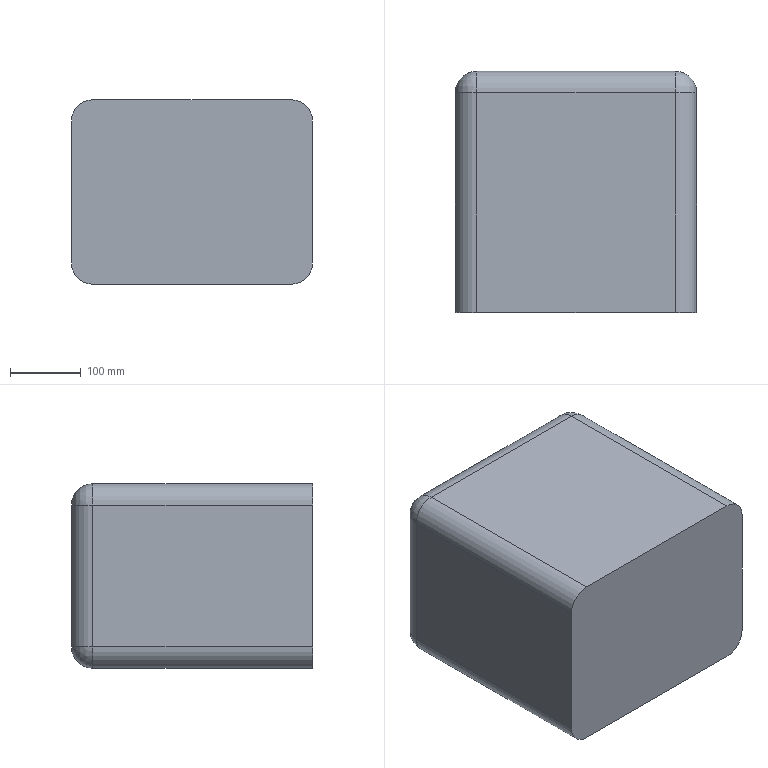Part | 1 solid | 18 faces | box 340 x 340 x 260 mm | volume 29579637 mm3 | cylinder 8 | plane 6 | sphere 4 | commonest cylinder face diameters 60 x8
STEP:
#1=CARTESIAN_POINT('',(170.,0.,100.));
#2=VERTEX_POINT('',#1);
#3=CARTESIAN_POINT('',(170.,0.,-100.));
#4=VERTEX_POINT('',#3);
#5=CARTESIAN_POINT('',(170.,0.,-130.));
#6=DIRECTION('',(0.,0.,-1.));
#7=VECTOR('',#6,1000.);
#8=LINE('',#5,#7);
#9=EDGE_CURVE('',#2,#4,#8,.T.);
#10=ORIENTED_EDGE('',*,*,#9,.T.);
#11=CARTESIAN_POINT('',(170.,310.,-100.));
#12=VERTEX_POINT('',#11);
#13=CARTESIAN_POINT('',(170.,340.,-100.));
#14=DIRECTION('',(0.,1.,0.));
#15=VECTOR('',#14,1000.);
#16=LINE('',#13,#15);
#17=EDGE_CURVE('',#4,#12,#16,.T.);
#18=ORIENTED_EDGE('',*,*,#17,.T.);
#19=CARTESIAN_POINT('',(170.,310.,100.));
#20=VERTEX_POINT('',#19);
#21=CARTESIAN_POINT('',(170.,310.,130.));
#22=DIRECTION('',(0.,0.,1.));
#23=VECTOR('',#22,1000.);
#24=LINE('',#21,#23);
#25=EDGE_CURVE('',#12,#20,#24,.T.);
#26=ORIENTED_EDGE('',*,*,#25,.T.);
#27=CARTESIAN_POINT('',(170.,340.,100.));
#28=DIRECTION('',(0.,-1.,0.));
#29=VECTOR('',#28,1000.);
#30=LINE('',#27,#29);
#31=EDGE_CURVE('',#20,#2,#30,.T.);
#32=ORIENTED_EDGE('',*,*,#31,.T.);
#33=EDGE_LOOP('',(#10,#18,#26,#32));
#34=FACE_OUTER_BOUND('',#33,.T.);
#35=CARTESIAN_POINT('',(170.,340.,-130.));
#36=DIRECTION('',(-1.,0.,0.));
#37=DIRECTION('',(0.,0.,1.));
#38=AXIS2_PLACEMENT_3D('',#35,#36,#37);
#39=PLANE('',#38);
#40=ADVANCED_FACE('',(#34),#39,.F.);
#41=CARTESIAN_POINT('',(140.,0.,-130.));
#42=VERTEX_POINT('',#41);
#43=CARTESIAN_POINT('',(-140.,0.,-130.));
#44=VERTEX_POINT('',#43);
#45=CARTESIAN_POINT('',(-170.,0.,-130.));
#46=DIRECTION('',(-1.,0.,0.));
#47=VECTOR('',#46,1000.);
#48=LINE('',#45,#47);
#49=EDGE_CURVE('',#42,#44,#48,.T.);
#50=ORIENTED_EDGE('',*,*,#49,.T.);
#51=CARTESIAN_POINT('',(-140.,310.,-130.));
#52=VERTEX_POINT('',#51);
#53=CARTESIAN_POINT('',(-140.,340.,-130.));
#54=DIRECTION('',(0.,1.,0.));
#55=VECTOR('',#54,1000.);
#56=LINE('',#53,#55);
#57=EDGE_CURVE('',#44,#52,#56,.T.);
#58=ORIENTED_EDGE('',*,*,#57,.T.);
#59=CARTESIAN_POINT('',(140.,310.,-130.));
#60=VERTEX_POINT('',#59);
#61=CARTESIAN_POINT('',(170.,310.,-130.));
#62=DIRECTION('',(1.,0.,0.));
#63=VECTOR('',#62,1000.);
#64=LINE('',#61,#63);
#65=EDGE_CURVE('',#52,#60,#64,.T.);
#66=ORIENTED_EDGE('',*,*,#65,.T.);
#67=CARTESIAN_POINT('',(140.,340.,-130.));
#68=DIRECTION('',(0.,-1.,0.));
#69=VECTOR('',#68,1000.);
#70=LINE('',#67,#69);
#71=EDGE_CURVE('',#60,#42,#70,.T.);
#72=ORIENTED_EDGE('',*,*,#71,.T.);
#73=EDGE_LOOP('',(#50,#58,#66,#72));
#74=FACE_OUTER_BOUND('',#73,.T.);
#75=CARTESIAN_POINT('',(-170.,340.,-130.));
#76=DIRECTION('',(0.,0.,1.));
#77=DIRECTION('',(1.,0.,0.));
#78=AXIS2_PLACEMENT_3D('',#75,#76,#77);
#79=PLANE('',#78);
#80=ADVANCED_FACE('',(#74),#79,.F.);
#81=CARTESIAN_POINT('',(-170.,310.,100.));
#82=VERTEX_POINT('',#81);
#83=CARTESIAN_POINT('',(-170.,310.,-100.));
#84=VERTEX_POINT('',#83);
#85=CARTESIAN_POINT('',(-170.,310.,-130.));
#86=DIRECTION('',(0.,0.,-1.));
#87=VECTOR('',#86,1000.);
#88=LINE('',#85,#87);
#89=EDGE_CURVE('',#82,#84,#88,.T.);
#90=ORIENTED_EDGE('',*,*,#89,.T.);
#91=CARTESIAN_POINT('',(-170.,0.,-100.));
#92=VERTEX_POINT('',#91);
#93=CARTESIAN_POINT('',(-170.,340.,-100.));
#94=DIRECTION('',(0.,-1.,0.));
#95=VECTOR('',#94,1000.);
#96=LINE('',#93,#95);
#97=EDGE_CURVE('',#84,#92,#96,.T.);
#98=ORIENTED_EDGE('',*,*,#97,.T.);
#99=CARTESIAN_POINT('',(-170.,0.,100.));
#100=VERTEX_POINT('',#99);
#101=CARTESIAN_POINT('',(-170.,0.,-130.));
#102=DIRECTION('',(0.,0.,1.));
#103=VECTOR('',#102,1000.);
#104=LINE('',#101,#103);
#105=EDGE_CURVE('',#92,#100,#104,.T.);
#106=ORIENTED_EDGE('',*,*,#105,.T.);
#107=CARTESIAN_POINT('',(-170.,340.,100.));
#108=DIRECTION('',(0.,1.,0.));
#109=VECTOR('',#108,1000.);
#110=LINE('',#107,#109);
#111=EDGE_CURVE('',#100,#82,#110,.T.);
#112=ORIENTED_EDGE('',*,*,#111,.T.);
#113=EDGE_LOOP('',(#90,#98,#106,#112));
#114=FACE_OUTER_BOUND('',#113,.T.);
#115=CARTESIAN_POINT('',(-170.,340.,-130.));
#116=DIRECTION('',(1.,0.,0.));
#117=DIRECTION('',(0.,0.,-1.));
#118=AXIS2_PLACEMENT_3D('',#115,#116,#117);
#119=PLANE('',#118);
#120=ADVANCED_FACE('',(#114),#119,.F.);
#121=CARTESIAN_POINT('',(140.,310.,130.));
#122=VERTEX_POINT('',#121);
#123=CARTESIAN_POINT('',(-140.,310.,130.));
#124=VERTEX_POINT('',#123);
#125=CARTESIAN_POINT('',(-170.,310.,130.));
#126=DIRECTION('',(-1.,0.,0.));
#127=VECTOR('',#126,1000.);
#128=LINE('',#125,#127);
#129=EDGE_CURVE('',#122,#124,#128,.T.);
#130=ORIENTED_EDGE('',*,*,#129,.T.);
#131=CARTESIAN_POINT('',(-140.,0.,130.));
#132=VERTEX_POINT('',#131);
#133=CARTESIAN_POINT('',(-140.,340.,130.));
#134=DIRECTION('',(0.,-1.,0.));
#135=VECTOR('',#134,1000.);
#136=LINE('',#133,#135);
#137=EDGE_CURVE('',#124,#132,#136,.T.);
#138=ORIENTED_EDGE('',*,*,#137,.T.);
#139=CARTESIAN_POINT('',(140.,0.,130.));
#140=VERTEX_POINT('',#139);
#141=CARTESIAN_POINT('',(-170.,0.,130.));
#142=DIRECTION('',(1.,0.,0.));
#143=VECTOR('',#142,1000.);
#144=LINE('',#141,#143);
#145=EDGE_CURVE('',#132,#140,#144,.T.);
#146=ORIENTED_EDGE('',*,*,#145,.T.);
#147=CARTESIAN_POINT('',(140.,340.,130.));
#148=DIRECTION('',(0.,1.,0.));
#149=VECTOR('',#148,1000.);
#150=LINE('',#147,#149);
#151=EDGE_CURVE('',#140,#122,#150,.T.);
#152=ORIENTED_EDGE('',*,*,#151,.T.);
#153=EDGE_LOOP('',(#130,#138,#146,#152));
#154=FACE_OUTER_BOUND('',#153,.T.);
#155=CARTESIAN_POINT('',(-170.,340.,130.));
#156=DIRECTION('',(0.,0.,-1.));
#157=DIRECTION('',(-1.,0.,0.));
#158=AXIS2_PLACEMENT_3D('',#155,#156,#157);
#159=PLANE('',#158);
#160=ADVANCED_FACE('',(#154),#159,.F.);
#161=CARTESIAN_POINT('',(140.,340.,100.));
#162=VERTEX_POINT('',#161);
#163=CARTESIAN_POINT('',(140.,340.,-100.));
#164=VERTEX_POINT('',#163);
#165=CARTESIAN_POINT('',(140.,340.,-130.));
#166=DIRECTION('',(0.,0.,-1.));
#167=VECTOR('',#166,1000.);
#168=LINE('',#165,#167);
#169=EDGE_CURVE('',#162,#164,#168,.T.);
#170=ORIENTED_EDGE('',*,*,#169,.T.);
#171=CARTESIAN_POINT('',(-140.,340.,-100.));
#172=VERTEX_POINT('',#171);
#173=CARTESIAN_POINT('',(-170.,340.,-100.));
#174=DIRECTION('',(-1.,0.,0.));
#175=VECTOR('',#174,1000.);
#176=LINE('',#173,#175);
#177=EDGE_CURVE('',#164,#172,#176,.T.);
#178=ORIENTED_EDGE('',*,*,#177,.T.);
#179=CARTESIAN_POINT('',(-140.,340.,100.));
#180=VERTEX_POINT('',#179);
#181=CARTESIAN_POINT('',(-140.,340.,130.));
#182=DIRECTION('',(0.,0.,1.));
#183=VECTOR('',#182,1000.);
#184=LINE('',#181,#183);
#185=EDGE_CURVE('',#172,#180,#184,.T.);
#186=ORIENTED_EDGE('',*,*,#185,.T.);
#187=CARTESIAN_POINT('',(170.,340.,100.));
#188=DIRECTION('',(1.,0.,0.));
#189=VECTOR('',#188,1000.);
#190=LINE('',#187,#189);
#191=EDGE_CURVE('',#180,#162,#190,.T.);
#192=ORIENTED_EDGE('',*,*,#191,.T.);
#193=EDGE_LOOP('',(#170,#178,#186,#192));
#194=FACE_OUTER_BOUND('',#193,.T.);
#195=CARTESIAN_POINT('',(0.,340.,0.));
#196=DIRECTION('',(0.,1.,0.));
#197=DIRECTION('',(0.,0.,1.));
#198=AXIS2_PLACEMENT_3D('',#195,#196,#197);
#199=PLANE('',#198);
#200=ADVANCED_FACE('',(#194),#199,.T.);
#201=ORIENTED_EDGE('',*,*,#105,.F.);
#202=CARTESIAN_POINT('',(-140.,0.,-100.));
#203=DIRECTION('',(0.,-1.,0.));
#204=DIRECTION('',(0.,0.,1.));
#205=AXIS2_PLACEMENT_3D('',#202,#203,#204);
#206=CIRCLE('',#205,30.);
#207=EDGE_CURVE('',#92,#44,#206,.T.);
#208=ORIENTED_EDGE('',*,*,#207,.T.);
#209=ORIENTED_EDGE('',*,*,#49,.F.);
#210=CARTESIAN_POINT('',(140.,0.,-100.));
#211=DIRECTION('',(0.,-1.,0.));
#212=DIRECTION('',(0.,0.,1.));
#213=AXIS2_PLACEMENT_3D('',#210,#211,#212);
#214=CIRCLE('',#213,30.);
#215=EDGE_CURVE('',#42,#4,#214,.T.);
#216=ORIENTED_EDGE('',*,*,#215,.T.);
#217=ORIENTED_EDGE('',*,*,#9,.F.);
#218=CARTESIAN_POINT('',(140.,0.,100.));
#219=DIRECTION('',(0.,-1.,0.));
#220=DIRECTION('',(0.,0.,1.));
#221=AXIS2_PLACEMENT_3D('',#218,#219,#220);
#222=CIRCLE('',#221,30.);
#223=EDGE_CURVE('',#2,#140,#222,.T.);
#224=ORIENTED_EDGE('',*,*,#223,.T.);
#225=ORIENTED_EDGE('',*,*,#145,.F.);
#226=CARTESIAN_POINT('',(-140.,0.,100.));
#227=DIRECTION('',(0.,-1.,0.));
#228=DIRECTION('',(0.,0.,1.));
#229=AXIS2_PLACEMENT_3D('',#226,#227,#228);
#230=CIRCLE('',#229,30.);
#231=EDGE_CURVE('',#132,#100,#230,.T.);
#232=ORIENTED_EDGE('',*,*,#231,.T.);
#233=EDGE_LOOP('',(#201,#208,#209,#216,#217,#224,#225,#232));
#234=FACE_OUTER_BOUND('',#233,.T.);
#235=CARTESIAN_POINT('',(0.,0.,0.));
#236=DIRECTION('',(0.,1.,0.));
#237=DIRECTION('',(0.,0.,1.));
#238=AXIS2_PLACEMENT_3D('',#235,#236,#237);
#239=PLANE('',#238);
#240=ADVANCED_FACE('',(#234),#239,.F.);
#241=CARTESIAN_POINT('',(140.,310.,100.));
#242=DIRECTION('',(0.,1.,0.));
#243=DIRECTION('',(0.,0.,1.));
#244=AXIS2_PLACEMENT_3D('',#241,#242,#243);
#245=CIRCLE('',#244,30.);
#246=EDGE_CURVE('',#122,#20,#245,.T.);
#247=ORIENTED_EDGE('',*,*,#246,.F.);
#248=ORIENTED_EDGE('',*,*,#151,.F.);
#249=ORIENTED_EDGE('',*,*,#223,.F.);
#250=ORIENTED_EDGE('',*,*,#31,.F.);
#251=EDGE_LOOP('',(#247,#248,#249,#250));
#252=FACE_OUTER_BOUND('',#251,.T.);
#253=CARTESIAN_POINT('',(140.,340.,100.));
#254=DIRECTION('',(0.,-1.,0.));
#255=DIRECTION('',(0.,0.,-1.));
#256=AXIS2_PLACEMENT_3D('',#253,#254,#255);
#257=CYLINDRICAL_SURFACE('',#256,30.);
#258=ADVANCED_FACE('',(#252),#257,.T.);
#259=CARTESIAN_POINT('',(140.,310.,100.));
#260=DIRECTION('',(-1.,0.,0.));
#261=DIRECTION('',(0.,0.,-1.));
#262=AXIS2_PLACEMENT_3D('',#259,#260,#261);
#263=CIRCLE('',#262,30.);
#264=EDGE_CURVE('',#122,#162,#263,.T.);
#265=ORIENTED_EDGE('',*,*,#264,.F.);
#266=ORIENTED_EDGE('',*,*,#246,.T.);
#267=CARTESIAN_POINT('',(140.,310.,100.));
#268=DIRECTION('',(0.,0.,-1.));
#269=DIRECTION('',(1.,0.,0.));
#270=AXIS2_PLACEMENT_3D('',#267,#268,#269);
#271=CIRCLE('',#270,30.);
#272=EDGE_CURVE('',#162,#20,#271,.T.);
#273=ORIENTED_EDGE('',*,*,#272,.F.);
#274=EDGE_LOOP('',(#265,#266,#273));
#275=FACE_OUTER_BOUND('',#274,.T.);
#276=CARTESIAN_POINT('',(140.,310.,100.));
#277=DIRECTION('',(0.,1.,0.));
#278=DIRECTION('',(1.,0.,0.));
#279=AXIS2_PLACEMENT_3D('',#276,#277,#278);
#280=SPHERICAL_SURFACE('',#279,30.);
#281=ADVANCED_FACE('',(#275),#280,.T.);
#282=ORIENTED_EDGE('',*,*,#215,.F.);
#283=ORIENTED_EDGE('',*,*,#71,.F.);
#284=CARTESIAN_POINT('',(140.,310.,-100.));
#285=DIRECTION('',(0.,1.,0.));
#286=DIRECTION('',(0.,0.,1.));
#287=AXIS2_PLACEMENT_3D('',#284,#285,#286);
#288=CIRCLE('',#287,30.);
#289=EDGE_CURVE('',#12,#60,#288,.T.);
#290=ORIENTED_EDGE('',*,*,#289,.F.);
#291=ORIENTED_EDGE('',*,*,#17,.F.);
#292=EDGE_LOOP('',(#282,#283,#290,#291));
#293=FACE_OUTER_BOUND('',#292,.T.);
#294=CARTESIAN_POINT('',(140.,340.,-100.));
#295=DIRECTION('',(0.,-1.,0.));
#296=DIRECTION('',(0.,0.,-1.));
#297=AXIS2_PLACEMENT_3D('',#294,#295,#296);
#298=CYLINDRICAL_SURFACE('',#297,30.);
#299=ADVANCED_FACE('',(#293),#298,.T.);
#300=ORIENTED_EDGE('',*,*,#272,.T.);
#301=ORIENTED_EDGE('',*,*,#25,.F.);
#302=CARTESIAN_POINT('',(140.,310.,-100.));
#303=DIRECTION('',(0.,0.,-1.));
#304=DIRECTION('',(-1.,0.,0.));
#305=AXIS2_PLACEMENT_3D('',#302,#303,#304);
#306=CIRCLE('',#305,30.);
#307=EDGE_CURVE('',#164,#12,#306,.T.);
#308=ORIENTED_EDGE('',*,*,#307,.F.);
#309=ORIENTED_EDGE('',*,*,#169,.F.);
#310=EDGE_LOOP('',(#300,#301,#308,#309));
#311=FACE_OUTER_BOUND('',#310,.T.);
#312=CARTESIAN_POINT('',(140.,310.,0.));
#313=DIRECTION('',(0.,0.,1.));
#314=DIRECTION('',(1.,0.,0.));
#315=AXIS2_PLACEMENT_3D('',#312,#313,#314);
#316=CYLINDRICAL_SURFACE('',#315,30.);
#317=ADVANCED_FACE('',(#311),#316,.T.);
#318=ORIENTED_EDGE('',*,*,#264,.T.);
#319=ORIENTED_EDGE('',*,*,#191,.F.);
#320=CARTESIAN_POINT('',(-140.,310.,100.));
#321=DIRECTION('',(-1.,0.,0.));
#322=DIRECTION('',(0.,0.,1.));
#323=AXIS2_PLACEMENT_3D('',#320,#321,#322);
#324=CIRCLE('',#323,30.);
#325=EDGE_CURVE('',#124,#180,#324,.T.);
#326=ORIENTED_EDGE('',*,*,#325,.F.);
#327=ORIENTED_EDGE('',*,*,#129,.F.);
#328=EDGE_LOOP('',(#318,#319,#326,#327));
#329=FACE_OUTER_BOUND('',#328,.T.);
#330=CARTESIAN_POINT('',(0.,310.,100.));
#331=DIRECTION('',(-1.,0.,0.));
#332=DIRECTION('',(0.,0.,1.));
#333=AXIS2_PLACEMENT_3D('',#330,#331,#332);
#334=CYLINDRICAL_SURFACE('',#333,30.);
#335=ADVANCED_FACE('',(#329),#334,.T.);
#336=ORIENTED_EDGE('',*,*,#231,.F.);
#337=ORIENTED_EDGE('',*,*,#137,.F.);
#338=CARTESIAN_POINT('',(-140.,310.,100.));
#339=DIRECTION('',(0.,1.,0.));
#340=DIRECTION('',(0.,0.,1.));
#341=AXIS2_PLACEMENT_3D('',#338,#339,#340);
#342=CIRCLE('',#341,30.);
#343=EDGE_CURVE('',#82,#124,#342,.T.);
#344=ORIENTED_EDGE('',*,*,#343,.F.);
#345=ORIENTED_EDGE('',*,*,#111,.F.);
#346=EDGE_LOOP('',(#336,#337,#344,#345));
#347=FACE_OUTER_BOUND('',#346,.T.);
#348=CARTESIAN_POINT('',(-140.,340.,100.));
#349=DIRECTION('',(0.,-1.,0.));
#350=DIRECTION('',(0.,0.,-1.));
#351=AXIS2_PLACEMENT_3D('',#348,#349,#350);
#352=CYLINDRICAL_SURFACE('',#351,30.);
#353=ADVANCED_FACE('',(#347),#352,.T.);
#354=ORIENTED_EDGE('',*,*,#307,.T.);
#355=ORIENTED_EDGE('',*,*,#289,.T.);
#356=CARTESIAN_POINT('',(140.,310.,-100.));
#357=DIRECTION('',(-1.,0.,0.));
#358=DIRECTION('',(0.,1.,0.));
#359=AXIS2_PLACEMENT_3D('',#356,#357,#358);
#360=CIRCLE('',#359,30.);
#361=EDGE_CURVE('',#164,#60,#360,.T.);
#362=ORIENTED_EDGE('',*,*,#361,.F.);
#363=EDGE_LOOP('',(#354,#355,#362));
#364=FACE_OUTER_BOUND('',#363,.T.);
#365=CARTESIAN_POINT('',(140.,310.,-100.));
#366=DIRECTION('',(0.,1.,0.));
#367=DIRECTION('',(1.,0.,0.));
#368=AXIS2_PLACEMENT_3D('',#365,#366,#367);
#369=SPHERICAL_SURFACE('',#368,30.);
#370=ADVANCED_FACE('',(#364),#369,.T.);
#371=ORIENTED_EDGE('',*,*,#343,.T.);
#372=ORIENTED_EDGE('',*,*,#325,.T.);
#373=CARTESIAN_POINT('',(-140.,310.,100.));
#374=DIRECTION('',(0.,0.,-1.));
#375=DIRECTION('',(1.,0.,0.));
#376=AXIS2_PLACEMENT_3D('',#373,#374,#375);
#377=CIRCLE('',#376,30.);
#378=EDGE_CURVE('',#82,#180,#377,.T.);
#379=ORIENTED_EDGE('',*,*,#378,.F.);
#380=EDGE_LOOP('',(#371,#372,#379));
#381=FACE_OUTER_BOUND('',#380,.T.);
#382=CARTESIAN_POINT('',(-140.,310.,100.));
#383=DIRECTION('',(0.,1.,0.));
#384=DIRECTION('',(1.,0.,0.));
#385=AXIS2_PLACEMENT_3D('',#382,#383,#384);
#386=SPHERICAL_SURFACE('',#385,30.);
#387=ADVANCED_FACE('',(#381),#386,.T.);
#388=ORIENTED_EDGE('',*,*,#361,.T.);
#389=ORIENTED_EDGE('',*,*,#65,.F.);
#390=CARTESIAN_POINT('',(-140.,310.,-100.));
#391=DIRECTION('',(-1.,0.,0.));
#392=DIRECTION('',(0.,0.,1.));
#393=AXIS2_PLACEMENT_3D('',#390,#391,#392);
#394=CIRCLE('',#393,30.);
#395=EDGE_CURVE('',#172,#52,#394,.T.);
#396=ORIENTED_EDGE('',*,*,#395,.F.);
#397=ORIENTED_EDGE('',*,*,#177,.F.);
#398=EDGE_LOOP('',(#388,#389,#396,#397));
#399=FACE_OUTER_BOUND('',#398,.T.);
#400=CARTESIAN_POINT('',(0.,310.,-100.));
#401=DIRECTION('',(1.,0.,0.));
#402=DIRECTION('',(0.,0.,-1.));
#403=AXIS2_PLACEMENT_3D('',#400,#401,#402);
#404=CYLINDRICAL_SURFACE('',#403,30.);
#405=ADVANCED_FACE('',(#399),#404,.T.);
#406=ORIENTED_EDGE('',*,*,#378,.T.);
#407=ORIENTED_EDGE('',*,*,#185,.F.);
#408=CARTESIAN_POINT('',(-140.,310.,-100.));
#409=DIRECTION('',(0.,0.,-1.));
#410=DIRECTION('',(-1.,0.,0.));
#411=AXIS2_PLACEMENT_3D('',#408,#409,#410);
#412=CIRCLE('',#411,30.);
#413=EDGE_CURVE('',#84,#172,#412,.T.);
#414=ORIENTED_EDGE('',*,*,#413,.F.);
#415=ORIENTED_EDGE('',*,*,#89,.F.);
#416=EDGE_LOOP('',(#406,#407,#414,#415));
#417=FACE_OUTER_BOUND('',#416,.T.);
#418=CARTESIAN_POINT('',(-140.,310.,0.));
#419=DIRECTION('',(0.,0.,-1.));
#420=DIRECTION('',(-1.,0.,0.));
#421=AXIS2_PLACEMENT_3D('',#418,#419,#420);
#422=CYLINDRICAL_SURFACE('',#421,30.);
#423=ADVANCED_FACE('',(#417),#422,.T.);
#424=ORIENTED_EDGE('',*,*,#413,.T.);
#425=ORIENTED_EDGE('',*,*,#395,.T.);
#426=CARTESIAN_POINT('',(-140.,310.,-100.));
#427=DIRECTION('',(0.,-1.,0.));
#428=DIRECTION('',(0.,0.,1.));
#429=AXIS2_PLACEMENT_3D('',#426,#427,#428);
#430=CIRCLE('',#429,30.);
#431=EDGE_CURVE('',#84,#52,#430,.T.);
#432=ORIENTED_EDGE('',*,*,#431,.F.);
#433=EDGE_LOOP('',(#424,#425,#432));
#434=FACE_OUTER_BOUND('',#433,.T.);
#435=CARTESIAN_POINT('',(-140.,310.,-100.));
#436=DIRECTION('',(0.,1.,0.));
#437=DIRECTION('',(1.,0.,0.));
#438=AXIS2_PLACEMENT_3D('',#435,#436,#437);
#439=SPHERICAL_SURFACE('',#438,30.);
#440=ADVANCED_FACE('',(#434),#439,.T.);
#441=ORIENTED_EDGE('',*,*,#431,.T.);
#442=ORIENTED_EDGE('',*,*,#57,.F.);
#443=ORIENTED_EDGE('',*,*,#207,.F.);
#444=ORIENTED_EDGE('',*,*,#97,.F.);
#445=EDGE_LOOP('',(#441,#442,#443,#444));
#446=FACE_OUTER_BOUND('',#445,.T.);
#447=CARTESIAN_POINT('',(-140.,340.,-100.));
#448=DIRECTION('',(0.,-1.,0.));
#449=DIRECTION('',(0.,0.,-1.));
#450=AXIS2_PLACEMENT_3D('',#447,#448,#449);
#451=CYLINDRICAL_SURFACE('',#450,30.);
#452=ADVANCED_FACE('',(#446),#451,.T.);
#453=CLOSED_SHELL('',(#40,#80,#120,#160,#200,#240,#258,#281,#299,#317,#335,#353,#370,#387,#405,#423,#440,#452));
#454=MANIFOLD_SOLID_BREP('',#453);
#455=CARTESIAN_POINT('',(0.,0.,0.));
#456=DIRECTION('',(0.,0.,1.));
#457=DIRECTION('',(1.,0.,0.));
#458=AXIS2_PLACEMENT_3D('',#455,#456,#457);
#459=(LENGTH_UNIT()NAMED_UNIT(*)SI_UNIT(.MILLI.,.METRE.));
#460=UNCERTAINTY_MEASURE_WITH_UNIT(LENGTH_MEASURE(0.00001),#459,'','');
#461=(NAMED_UNIT(*)PLANE_ANGLE_UNIT()SI_UNIT($,.RADIAN.));
#462=(NAMED_UNIT(*)SI_UNIT($,.STERADIAN.)SOLID_ANGLE_UNIT());
#463=(GEOMETRIC_REPRESENTATION_CONTEXT(3)GLOBAL_UNCERTAINTY_ASSIGNED_CONTEXT((#460))GLOBAL_UNIT_ASSIGNED_CONTEXT((#459,#461,#462))REPRESENTATION_CONTEXT('',''));
#464=ADVANCED_BREP_SHAPE_REPRESENTATION('',(#454,#458),#463);